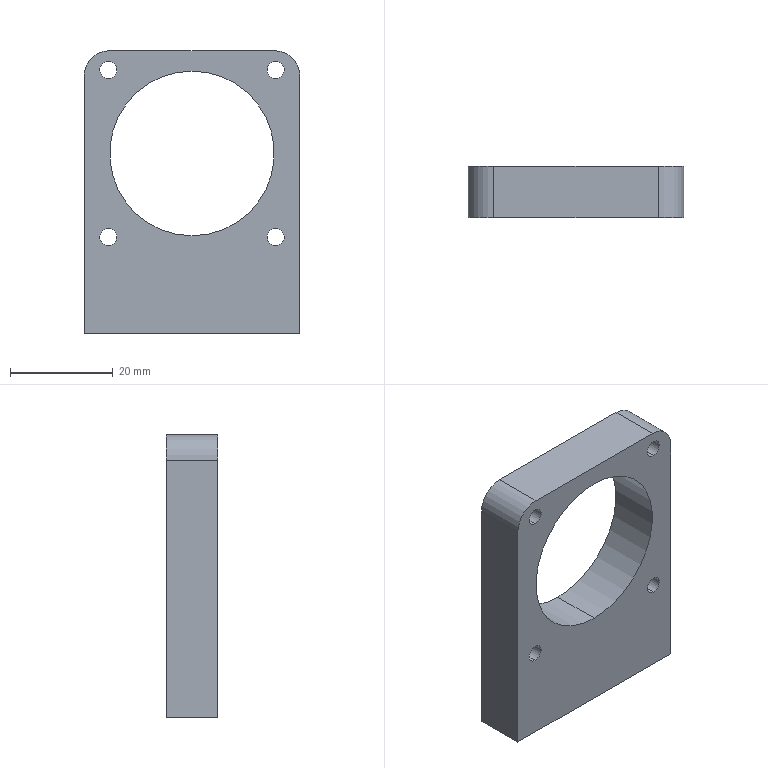Part | 1 solid | 26 faces | box 42 x 10 x 55 mm | volume 14397 mm3 | cylinder 16 | plane 6 | cone 4 | commonest cylinder face diameters 3.3 x12 10 x2 32 x2
STEP:
#1=CARTESIAN_POINT('',(-16.265,-5.,-18.915));
#2=VERTEX_POINT('',#1);
#3=CARTESIAN_POINT('',(-16.265,-5.,-15.615));
#4=VERTEX_POINT('',#3);
#5=CARTESIAN_POINT('',(-16.265,-5.,-17.265));
#6=DIRECTION('',(0.,1.,0.));
#7=DIRECTION('',(0.,0.,1.));
#8=AXIS2_PLACEMENT_3D('',#5,#6,#7);
#9=CIRCLE('',#8,1.65);
#10=EDGE_CURVE('',#2,#4,#9,.T.);
#11=ORIENTED_EDGE('',*,*,#10,.F.);
#12=CARTESIAN_POINT('',(-16.265,5.,-18.915));
#13=VERTEX_POINT('',#12);
#14=CARTESIAN_POINT('',(-16.265,5.,-18.915));
#15=DIRECTION('',(0.,1.,0.));
#16=VECTOR('',#15,1000.);
#17=LINE('',#14,#16);
#18=EDGE_CURVE('',#2,#13,#17,.T.);
#19=ORIENTED_EDGE('',*,*,#18,.T.);
#20=CARTESIAN_POINT('',(-16.265,5.,-15.615));
#21=VERTEX_POINT('',#20);
#22=CARTESIAN_POINT('',(-16.265,5.,-17.265));
#23=DIRECTION('',(0.,1.,0.));
#24=DIRECTION('',(0.,0.,1.));
#25=AXIS2_PLACEMENT_3D('',#22,#23,#24);
#26=CIRCLE('',#25,1.65);
#27=EDGE_CURVE('',#13,#21,#26,.T.);
#28=ORIENTED_EDGE('',*,*,#27,.T.);
#29=CARTESIAN_POINT('',(-16.265,5.,-15.615));
#30=DIRECTION('',(0.,1.,0.));
#31=VECTOR('',#30,1000.);
#32=LINE('',#29,#31);
#33=EDGE_CURVE('',#4,#21,#32,.T.);
#34=ORIENTED_EDGE('',*,*,#33,.F.);
#35=EDGE_LOOP('',(#11,#19,#28,#34));
#36=FACE_OUTER_BOUND('',#35,.T.);
#37=CARTESIAN_POINT('',(-16.265,5.,-17.265));
#38=DIRECTION('',(0.,1.,0.));
#39=DIRECTION('',(0.,0.,1.));
#40=AXIS2_PLACEMENT_3D('',#37,#38,#39);
#41=CYLINDRICAL_SURFACE('',#40,1.65);
#42=ADVANCED_FACE('',(#36),#41,.F.);
#43=CARTESIAN_POINT('',(16.265,-5.,-18.915));
#44=VERTEX_POINT('',#43);
#45=CARTESIAN_POINT('',(16.265,-5.,-15.615));
#46=VERTEX_POINT('',#45);
#47=CARTESIAN_POINT('',(16.265,-5.,-17.265));
#48=DIRECTION('',(0.,1.,0.));
#49=DIRECTION('',(0.,0.,1.));
#50=AXIS2_PLACEMENT_3D('',#47,#48,#49);
#51=CIRCLE('',#50,1.65);
#52=EDGE_CURVE('',#44,#46,#51,.T.);
#53=ORIENTED_EDGE('',*,*,#52,.F.);
#54=CARTESIAN_POINT('',(16.265,5.,-18.915));
#55=VERTEX_POINT('',#54);
#56=CARTESIAN_POINT('',(16.265,5.,-18.915));
#57=DIRECTION('',(0.,1.,0.));
#58=VECTOR('',#57,1000.);
#59=LINE('',#56,#58);
#60=EDGE_CURVE('',#44,#55,#59,.T.);
#61=ORIENTED_EDGE('',*,*,#60,.T.);
#62=CARTESIAN_POINT('',(16.265,5.,-15.615));
#63=VERTEX_POINT('',#62);
#64=CARTESIAN_POINT('',(16.265,5.,-17.265));
#65=DIRECTION('',(0.,1.,0.));
#66=DIRECTION('',(0.,0.,1.));
#67=AXIS2_PLACEMENT_3D('',#64,#65,#66);
#68=CIRCLE('',#67,1.65);
#69=EDGE_CURVE('',#55,#63,#68,.T.);
#70=ORIENTED_EDGE('',*,*,#69,.T.);
#71=CARTESIAN_POINT('',(16.265,5.,-15.615));
#72=DIRECTION('',(0.,1.,0.));
#73=VECTOR('',#72,1000.);
#74=LINE('',#71,#73);
#75=EDGE_CURVE('',#46,#63,#74,.T.);
#76=ORIENTED_EDGE('',*,*,#75,.F.);
#77=EDGE_LOOP('',(#53,#61,#70,#76));
#78=FACE_OUTER_BOUND('',#77,.T.);
#79=CARTESIAN_POINT('',(16.265,5.,-17.265));
#80=DIRECTION('',(0.,1.,0.));
#81=DIRECTION('',(0.,0.,1.));
#82=AXIS2_PLACEMENT_3D('',#79,#80,#81);
#83=CYLINDRICAL_SURFACE('',#82,1.65);
#84=ADVANCED_FACE('',(#78),#83,.F.);
#85=CARTESIAN_POINT('',(-16.265,-5.,13.615));
#86=VERTEX_POINT('',#85);
#87=CARTESIAN_POINT('',(-16.265,-5.,16.915));
#88=VERTEX_POINT('',#87);
#89=CARTESIAN_POINT('',(-16.265,-5.,15.265));
#90=DIRECTION('',(0.,1.,0.));
#91=DIRECTION('',(0.,0.,1.));
#92=AXIS2_PLACEMENT_3D('',#89,#90,#91);
#93=CIRCLE('',#92,1.65);
#94=EDGE_CURVE('',#86,#88,#93,.T.);
#95=ORIENTED_EDGE('',*,*,#94,.F.);
#96=CARTESIAN_POINT('',(-16.265,5.,13.615));
#97=VERTEX_POINT('',#96);
#98=CARTESIAN_POINT('',(-16.265,5.,13.615));
#99=DIRECTION('',(0.,1.,0.));
#100=VECTOR('',#99,1000.);
#101=LINE('',#98,#100);
#102=EDGE_CURVE('',#86,#97,#101,.T.);
#103=ORIENTED_EDGE('',*,*,#102,.T.);
#104=CARTESIAN_POINT('',(-16.265,5.,16.915));
#105=VERTEX_POINT('',#104);
#106=CARTESIAN_POINT('',(-16.265,5.,15.265));
#107=DIRECTION('',(0.,1.,0.));
#108=DIRECTION('',(0.,0.,1.));
#109=AXIS2_PLACEMENT_3D('',#106,#107,#108);
#110=CIRCLE('',#109,1.65);
#111=EDGE_CURVE('',#97,#105,#110,.T.);
#112=ORIENTED_EDGE('',*,*,#111,.T.);
#113=CARTESIAN_POINT('',(-16.265,5.,16.915));
#114=DIRECTION('',(0.,1.,0.));
#115=VECTOR('',#114,1000.);
#116=LINE('',#113,#115);
#117=EDGE_CURVE('',#88,#105,#116,.T.);
#118=ORIENTED_EDGE('',*,*,#117,.F.);
#119=EDGE_LOOP('',(#95,#103,#112,#118));
#120=FACE_OUTER_BOUND('',#119,.T.);
#121=CARTESIAN_POINT('',(-16.265,5.,15.265));
#122=DIRECTION('',(0.,1.,0.));
#123=DIRECTION('',(0.,0.,1.));
#124=AXIS2_PLACEMENT_3D('',#121,#122,#123);
#125=CYLINDRICAL_SURFACE('',#124,1.65);
#126=ADVANCED_FACE('',(#120),#125,.F.);
#127=CARTESIAN_POINT('',(16.265,-5.,13.615));
#128=VERTEX_POINT('',#127);
#129=CARTESIAN_POINT('',(16.265,-5.,16.915));
#130=VERTEX_POINT('',#129);
#131=CARTESIAN_POINT('',(16.265,-5.,15.265));
#132=DIRECTION('',(0.,1.,0.));
#133=DIRECTION('',(0.,0.,1.));
#134=AXIS2_PLACEMENT_3D('',#131,#132,#133);
#135=CIRCLE('',#134,1.65);
#136=EDGE_CURVE('',#128,#130,#135,.T.);
#137=ORIENTED_EDGE('',*,*,#136,.F.);
#138=CARTESIAN_POINT('',(16.265,5.,13.615));
#139=VERTEX_POINT('',#138);
#140=CARTESIAN_POINT('',(16.265,5.,13.615));
#141=DIRECTION('',(0.,1.,0.));
#142=VECTOR('',#141,1000.);
#143=LINE('',#140,#142);
#144=EDGE_CURVE('',#128,#139,#143,.T.);
#145=ORIENTED_EDGE('',*,*,#144,.T.);
#146=CARTESIAN_POINT('',(16.265,5.,16.915));
#147=VERTEX_POINT('',#146);
#148=CARTESIAN_POINT('',(16.265,5.,15.265));
#149=DIRECTION('',(0.,1.,0.));
#150=DIRECTION('',(0.,0.,1.));
#151=AXIS2_PLACEMENT_3D('',#148,#149,#150);
#152=CIRCLE('',#151,1.65);
#153=EDGE_CURVE('',#139,#147,#152,.T.);
#154=ORIENTED_EDGE('',*,*,#153,.T.);
#155=CARTESIAN_POINT('',(16.265,5.,16.915));
#156=DIRECTION('',(0.,1.,0.));
#157=VECTOR('',#156,1000.);
#158=LINE('',#155,#157);
#159=EDGE_CURVE('',#130,#147,#158,.T.);
#160=ORIENTED_EDGE('',*,*,#159,.F.);
#161=EDGE_LOOP('',(#137,#145,#154,#160));
#162=FACE_OUTER_BOUND('',#161,.T.);
#163=CARTESIAN_POINT('',(16.265,5.,15.265));
#164=DIRECTION('',(0.,1.,0.));
#165=DIRECTION('',(0.,0.,1.));
#166=AXIS2_PLACEMENT_3D('',#163,#164,#165);
#167=CYLINDRICAL_SURFACE('',#166,1.65);
#168=ADVANCED_FACE('',(#162),#167,.F.);
#169=CARTESIAN_POINT('',(0.,-5.,-17.));
#170=VERTEX_POINT('',#169);
#171=CARTESIAN_POINT('',(0.,-5.,15.));
#172=VERTEX_POINT('',#171);
#173=CARTESIAN_POINT('',(0.,-5.,-1.));
#174=DIRECTION('',(0.,1.,0.));
#175=DIRECTION('',(0.,0.,1.));
#176=AXIS2_PLACEMENT_3D('',#173,#174,#175);
#177=CIRCLE('',#176,16.);
#178=EDGE_CURVE('',#170,#172,#177,.T.);
#179=ORIENTED_EDGE('',*,*,#178,.F.);
#180=CARTESIAN_POINT('',(0.,5.,-17.));
#181=VERTEX_POINT('',#180);
#182=CARTESIAN_POINT('',(0.,-5.,-17.));
#183=DIRECTION('',(0.,1.,0.));
#184=VECTOR('',#183,1000.);
#185=LINE('',#182,#184);
#186=EDGE_CURVE('',#170,#181,#185,.T.);
#187=ORIENTED_EDGE('',*,*,#186,.T.);
#188=CARTESIAN_POINT('',(0.,5.,15.));
#189=VERTEX_POINT('',#188);
#190=CARTESIAN_POINT('',(0.,5.,-1.));
#191=DIRECTION('',(0.,1.,0.));
#192=DIRECTION('',(0.,0.,1.));
#193=AXIS2_PLACEMENT_3D('',#190,#191,#192);
#194=CIRCLE('',#193,16.);
#195=EDGE_CURVE('',#181,#189,#194,.T.);
#196=ORIENTED_EDGE('',*,*,#195,.T.);
#197=CARTESIAN_POINT('',(0.,-5.,15.));
#198=DIRECTION('',(0.,1.,0.));
#199=VECTOR('',#198,1000.);
#200=LINE('',#197,#199);
#201=EDGE_CURVE('',#172,#189,#200,.T.);
#202=ORIENTED_EDGE('',*,*,#201,.F.);
#203=EDGE_LOOP('',(#179,#187,#196,#202));
#204=FACE_OUTER_BOUND('',#203,.T.);
#205=CARTESIAN_POINT('',(0.,-5.,-1.));
#206=DIRECTION('',(0.,1.,0.));
#207=DIRECTION('',(0.,0.,1.));
#208=AXIS2_PLACEMENT_3D('',#205,#206,#207);
#209=CYLINDRICAL_SURFACE('',#208,16.);
#210=ADVANCED_FACE('',(#204),#209,.F.);
#211=CARTESIAN_POINT('',(16.65,0.,-24.));
#212=VERTEX_POINT('',#211);
#213=CARTESIAN_POINT('',(13.35,0.,-24.));
#214=VERTEX_POINT('',#213);
#215=CARTESIAN_POINT('',(15.,0.,-24.));
#216=DIRECTION('',(0.,0.,-1.));
#217=DIRECTION('',(-1.,0.,0.));
#218=AXIS2_PLACEMENT_3D('',#215,#216,#217);
#219=CIRCLE('',#218,1.65);
#220=EDGE_CURVE('',#212,#214,#219,.T.);
#221=ORIENTED_EDGE('',*,*,#220,.F.);
#222=CARTESIAN_POINT('',(16.65,0.,-36.));
#223=VERTEX_POINT('',#222);
#224=CARTESIAN_POINT('',(16.65,0.,-36.));
#225=DIRECTION('',(0.,0.,-1.));
#226=VECTOR('',#225,1000.);
#227=LINE('',#224,#226);
#228=EDGE_CURVE('',#212,#223,#227,.T.);
#229=ORIENTED_EDGE('',*,*,#228,.T.);
#230=CARTESIAN_POINT('',(13.35,0.,-36.));
#231=VERTEX_POINT('',#230);
#232=CARTESIAN_POINT('',(15.,0.,-36.));
#233=DIRECTION('',(0.,0.,-1.));
#234=DIRECTION('',(-1.,0.,0.));
#235=AXIS2_PLACEMENT_3D('',#232,#233,#234);
#236=CIRCLE('',#235,1.65);
#237=EDGE_CURVE('',#223,#231,#236,.T.);
#238=ORIENTED_EDGE('',*,*,#237,.T.);
#239=CARTESIAN_POINT('',(13.35,0.,-36.));
#240=DIRECTION('',(0.,0.,-1.));
#241=VECTOR('',#240,1000.);
#242=LINE('',#239,#241);
#243=EDGE_CURVE('',#214,#231,#242,.T.);
#244=ORIENTED_EDGE('',*,*,#243,.F.);
#245=EDGE_LOOP('',(#221,#229,#238,#244));
#246=FACE_OUTER_BOUND('',#245,.T.);
#247=CARTESIAN_POINT('',(15.,0.,-36.));
#248=DIRECTION('',(0.,0.,-1.));
#249=DIRECTION('',(-1.,0.,0.));
#250=AXIS2_PLACEMENT_3D('',#247,#248,#249);
#251=CYLINDRICAL_SURFACE('',#250,1.65);
#252=ADVANCED_FACE('',(#246),#251,.F.);
#253=CARTESIAN_POINT('',(15.,0.,-23.009));
#254=VERTEX_POINT('',#253);
#255=CARTESIAN_POINT('',(13.35,0.,-24.));
#256=DIRECTION('',(-0.8572,0.,-0.515));
#257=VECTOR('',#256,1000.);
#258=LINE('',#255,#257);
#259=EDGE_CURVE('',#254,#214,#258,.T.);
#260=ORIENTED_EDGE('',*,*,#259,.F.);
#261=CARTESIAN_POINT('',(16.65,0.,-24.));
#262=DIRECTION('',(0.8572,0.,-0.515));
#263=VECTOR('',#262,1000.);
#264=LINE('',#261,#263);
#265=EDGE_CURVE('',#254,#212,#264,.T.);
#266=ORIENTED_EDGE('',*,*,#265,.T.);
#267=ORIENTED_EDGE('',*,*,#220,.T.);
#268=EDGE_LOOP('',(#260,#266,#267));
#269=FACE_OUTER_BOUND('',#268,.T.);
#270=CARTESIAN_POINT('',(15.,0.,-24.));
#271=DIRECTION('',(0.,0.,-1.));
#272=DIRECTION('',(-1.,0.,0.));
#273=AXIS2_PLACEMENT_3D('',#270,#271,#272);
#274=CONICAL_SURFACE('',#273,1.65,1.03);
#275=ADVANCED_FACE('',(#269),#274,.F.);
#276=CARTESIAN_POINT('',(-13.35,0.,-24.));
#277=VERTEX_POINT('',#276);
#278=CARTESIAN_POINT('',(-16.65,0.,-24.));
#279=VERTEX_POINT('',#278);
#280=CARTESIAN_POINT('',(-15.,0.,-24.));
#281=DIRECTION('',(0.,0.,-1.));
#282=DIRECTION('',(-1.,0.,0.));
#283=AXIS2_PLACEMENT_3D('',#280,#281,#282);
#284=CIRCLE('',#283,1.65);
#285=EDGE_CURVE('',#277,#279,#284,.T.);
#286=ORIENTED_EDGE('',*,*,#285,.F.);
#287=CARTESIAN_POINT('',(-13.35,0.,-36.));
#288=VERTEX_POINT('',#287);
#289=CARTESIAN_POINT('',(-13.35,0.,-36.));
#290=DIRECTION('',(0.,0.,-1.));
#291=VECTOR('',#290,1000.);
#292=LINE('',#289,#291);
#293=EDGE_CURVE('',#277,#288,#292,.T.);
#294=ORIENTED_EDGE('',*,*,#293,.T.);
#295=CARTESIAN_POINT('',(-16.65,0.,-36.));
#296=VERTEX_POINT('',#295);
#297=CARTESIAN_POINT('',(-15.,0.,-36.));
#298=DIRECTION('',(0.,0.,-1.));
#299=DIRECTION('',(-1.,0.,0.));
#300=AXIS2_PLACEMENT_3D('',#297,#298,#299);
#301=CIRCLE('',#300,1.65);
#302=EDGE_CURVE('',#288,#296,#301,.T.);
#303=ORIENTED_EDGE('',*,*,#302,.T.);
#304=CARTESIAN_POINT('',(-16.65,0.,-36.));
#305=DIRECTION('',(0.,0.,-1.));
#306=VECTOR('',#305,1000.);
#307=LINE('',#304,#306);
#308=EDGE_CURVE('',#279,#296,#307,.T.);
#309=ORIENTED_EDGE('',*,*,#308,.F.);
#310=EDGE_LOOP('',(#286,#294,#303,#309));
#311=FACE_OUTER_BOUND('',#310,.T.);
#312=CARTESIAN_POINT('',(-15.,0.,-36.));
#313=DIRECTION('',(0.,0.,-1.));
#314=DIRECTION('',(-1.,0.,0.));
#315=AXIS2_PLACEMENT_3D('',#312,#313,#314);
#316=CYLINDRICAL_SURFACE('',#315,1.65);
#317=ADVANCED_FACE('',(#311),#316,.F.);
#318=CARTESIAN_POINT('',(-15.,0.,-23.009));
#319=VERTEX_POINT('',#318);
#320=CARTESIAN_POINT('',(-16.65,0.,-24.));
#321=DIRECTION('',(-0.8572,0.,-0.515));
#322=VECTOR('',#321,1000.);
#323=LINE('',#320,#322);
#324=EDGE_CURVE('',#319,#279,#323,.T.);
#325=ORIENTED_EDGE('',*,*,#324,.F.);
#326=CARTESIAN_POINT('',(-13.35,0.,-24.));
#327=DIRECTION('',(0.8572,0.,-0.515));
#328=VECTOR('',#327,1000.);
#329=LINE('',#326,#328);
#330=EDGE_CURVE('',#319,#277,#329,.T.);
#331=ORIENTED_EDGE('',*,*,#330,.T.);
#332=ORIENTED_EDGE('',*,*,#285,.T.);
#333=EDGE_LOOP('',(#325,#331,#332));
#334=FACE_OUTER_BOUND('',#333,.T.);
#335=CARTESIAN_POINT('',(-15.,0.,-24.));
#336=DIRECTION('',(0.,0.,-1.));
#337=DIRECTION('',(-1.,0.,0.));
#338=AXIS2_PLACEMENT_3D('',#335,#336,#337);
#339=CONICAL_SURFACE('',#338,1.65,1.03);
#340=ADVANCED_FACE('',(#334),#339,.F.);
#341=CARTESIAN_POINT('',(21.,5.,14.));
#342=VERTEX_POINT('',#341);
#343=CARTESIAN_POINT('',(21.,5.,-36.));
#344=VERTEX_POINT('',#343);
#345=CARTESIAN_POINT('',(21.,5.,-36.));
#346=DIRECTION('',(0.,0.,-1.));
#347=VECTOR('',#346,1000.);
#348=LINE('',#345,#347);
#349=EDGE_CURVE('',#342,#344,#348,.T.);
#350=ORIENTED_EDGE('',*,*,#349,.F.);
#351=CARTESIAN_POINT('',(21.,-5.,14.));
#352=VERTEX_POINT('',#351);
#353=CARTESIAN_POINT('',(21.,5.,14.));
#354=DIRECTION('',(0.,-1.,0.));
#355=VECTOR('',#354,1000.);
#356=LINE('',#353,#355);
#357=EDGE_CURVE('',#342,#352,#356,.T.);
#358=ORIENTED_EDGE('',*,*,#357,.T.);
#359=CARTESIAN_POINT('',(21.,-5.,-36.));
#360=VERTEX_POINT('',#359);
#361=CARTESIAN_POINT('',(21.,-5.,-36.));
#362=DIRECTION('',(0.,0.,-1.));
#363=VECTOR('',#362,1000.);
#364=LINE('',#361,#363);
#365=EDGE_CURVE('',#352,#360,#364,.T.);
#366=ORIENTED_EDGE('',*,*,#365,.T.);
#367=CARTESIAN_POINT('',(21.,5.,-36.));
#368=DIRECTION('',(0.,-1.,0.));
#369=VECTOR('',#368,1000.);
#370=LINE('',#367,#369);
#371=EDGE_CURVE('',#344,#360,#370,.T.);
#372=ORIENTED_EDGE('',*,*,#371,.F.);
#373=EDGE_LOOP('',(#350,#358,#366,#372));
#374=FACE_OUTER_BOUND('',#373,.T.);
#375=CARTESIAN_POINT('',(21.,5.,-36.));
#376=DIRECTION('',(-1.,0.,0.));
#377=DIRECTION('',(0.,0.,1.));
#378=AXIS2_PLACEMENT_3D('',#375,#376,#377);
#379=PLANE('',#378);
#380=ADVANCED_FACE('',(#374),#379,.F.);
#381=CARTESIAN_POINT('',(15.,0.,-36.));
#382=DIRECTION('',(0.,0.,-1.));
#383=DIRECTION('',(-1.,0.,0.));
#384=AXIS2_PLACEMENT_3D('',#381,#382,#383);
#385=CIRCLE('',#384,1.65);
#386=EDGE_CURVE('',#231,#223,#385,.T.);
#387=ORIENTED_EDGE('',*,*,#386,.F.);
#388=ORIENTED_EDGE('',*,*,#237,.F.);
#389=EDGE_LOOP('',(#387,#388));
#390=FACE_BOUND('',#389,.T.);
#391=CARTESIAN_POINT('',(-15.,0.,-36.));
#392=DIRECTION('',(0.,0.,-1.));
#393=DIRECTION('',(-1.,0.,0.));
#394=AXIS2_PLACEMENT_3D('',#391,#392,#393);
#395=CIRCLE('',#394,1.65);
#396=EDGE_CURVE('',#296,#288,#395,.T.);
#397=ORIENTED_EDGE('',*,*,#396,.F.);
#398=ORIENTED_EDGE('',*,*,#302,.F.);
#399=EDGE_LOOP('',(#397,#398));
#400=FACE_BOUND('',#399,.T.);
#401=CARTESIAN_POINT('',(-21.,-5.,-36.));
#402=VERTEX_POINT('',#401);
#403=CARTESIAN_POINT('',(-21.,-5.,-36.));
#404=DIRECTION('',(-1.,0.,0.));
#405=VECTOR('',#404,1000.);
#406=LINE('',#403,#405);
#407=EDGE_CURVE('',#360,#402,#406,.T.);
#408=ORIENTED_EDGE('',*,*,#407,.T.);
#409=CARTESIAN_POINT('',(-21.,5.,-36.));
#410=VERTEX_POINT('',#409);
#411=CARTESIAN_POINT('',(-21.,5.,-36.));
#412=DIRECTION('',(0.,-1.,0.));
#413=VECTOR('',#412,1000.);
#414=LINE('',#411,#413);
#415=EDGE_CURVE('',#410,#402,#414,.T.);
#416=ORIENTED_EDGE('',*,*,#415,.F.);
#417=CARTESIAN_POINT('',(-21.,5.,-36.));
#418=DIRECTION('',(-1.,0.,0.));
#419=VECTOR('',#418,1000.);
#420=LINE('',#417,#419);
#421=EDGE_CURVE('',#344,#410,#420,.T.);
#422=ORIENTED_EDGE('',*,*,#421,.F.);
#423=ORIENTED_EDGE('',*,*,#371,.T.);
#424=EDGE_LOOP('',(#408,#416,#422,#423));
#425=FACE_OUTER_BOUND('',#424,.T.);
#426=CARTESIAN_POINT('',(-21.,5.,-36.));
#427=DIRECTION('',(0.,0.,1.));
#428=DIRECTION('',(1.,0.,0.));
#429=AXIS2_PLACEMENT_3D('',#426,#427,#428);
#430=PLANE('',#429);
#431=ADVANCED_FACE('',(#390,#400,#425),#430,.F.);
#432=CARTESIAN_POINT('',(-21.,-5.,14.));
#433=VERTEX_POINT('',#432);
#434=CARTESIAN_POINT('',(-21.,-5.,-36.));
#435=DIRECTION('',(0.,0.,1.));
#436=VECTOR('',#435,1000.);
#437=LINE('',#434,#436);
#438=EDGE_CURVE('',#402,#433,#437,.T.);
#439=ORIENTED_EDGE('',*,*,#438,.T.);
#440=CARTESIAN_POINT('',(-21.,5.,14.));
#441=VERTEX_POINT('',#440);
#442=CARTESIAN_POINT('',(-21.,5.,14.));
#443=DIRECTION('',(0.,1.,0.));
#444=VECTOR('',#443,1000.);
#445=LINE('',#442,#444);
#446=EDGE_CURVE('',#433,#441,#445,.T.);
#447=ORIENTED_EDGE('',*,*,#446,.T.);
#448=CARTESIAN_POINT('',(-21.,5.,-36.));
#449=DIRECTION('',(0.,0.,1.));
#450=VECTOR('',#449,1000.);
#451=LINE('',#448,#450);
#452=EDGE_CURVE('',#410,#441,#451,.T.);
#453=ORIENTED_EDGE('',*,*,#452,.F.);
#454=ORIENTED_EDGE('',*,*,#415,.T.);
#455=EDGE_LOOP('',(#439,#447,#453,#454));
#456=FACE_OUTER_BOUND('',#455,.T.);
#457=CARTESIAN_POINT('',(-21.,5.,-36.));
#458=DIRECTION('',(1.,0.,0.));
#459=DIRECTION('',(0.,0.,-1.));
#460=AXIS2_PLACEMENT_3D('',#457,#458,#459);
#461=PLANE('',#460);
#462=ADVANCED_FACE('',(#456),#461,.F.);
#463=CARTESIAN_POINT('',(-16.265,5.,-17.265));
#464=DIRECTION('',(0.,1.,0.));
#465=DIRECTION('',(0.,0.,1.));
#466=AXIS2_PLACEMENT_3D('',#463,#464,#465);
#467=CIRCLE('',#466,1.65);
#468=EDGE_CURVE('',#21,#13,#467,.T.);
#469=ORIENTED_EDGE('',*,*,#468,.F.);
#470=ORIENTED_EDGE('',*,*,#27,.F.);
#471=EDGE_LOOP('',(#469,#470));
#472=FACE_BOUND('',#471,.T.);
#473=CARTESIAN_POINT('',(16.265,5.,-17.265));
#474=DIRECTION('',(0.,1.,0.));
#475=DIRECTION('',(0.,0.,1.));
#476=AXIS2_PLACEMENT_3D('',#473,#474,#475);
#477=CIRCLE('',#476,1.65);
#478=EDGE_CURVE('',#63,#55,#477,.T.);
#479=ORIENTED_EDGE('',*,*,#478,.F.);
#480=ORIENTED_EDGE('',*,*,#69,.F.);
#481=EDGE_LOOP('',(#479,#480));
#482=FACE_BOUND('',#481,.T.);
#483=CARTESIAN_POINT('',(-16.265,5.,15.265));
#484=DIRECTION('',(0.,1.,0.));
#485=DIRECTION('',(0.,0.,1.));
#486=AXIS2_PLACEMENT_3D('',#483,#484,#485);
#487=CIRCLE('',#486,1.65);
#488=EDGE_CURVE('',#105,#97,#487,.T.);
#489=ORIENTED_EDGE('',*,*,#488,.F.);
#490=ORIENTED_EDGE('',*,*,#111,.F.);
#491=EDGE_LOOP('',(#489,#490));
#492=FACE_BOUND('',#491,.T.);
#493=CARTESIAN_POINT('',(16.265,5.,15.265));
#494=DIRECTION('',(0.,1.,0.));
#495=DIRECTION('',(0.,0.,1.));
#496=AXIS2_PLACEMENT_3D('',#493,#494,#495);
#497=CIRCLE('',#496,1.65);
#498=EDGE_CURVE('',#147,#139,#497,.T.);
#499=ORIENTED_EDGE('',*,*,#498,.F.);
#500=ORIENTED_EDGE('',*,*,#153,.F.);
#501=EDGE_LOOP('',(#499,#500));
#502=FACE_BOUND('',#501,.T.);
#503=ORIENTED_EDGE('',*,*,#452,.T.);
#504=CARTESIAN_POINT('',(-16.,5.,19.));
#505=VERTEX_POINT('',#504);
#506=CARTESIAN_POINT('',(-16.,5.,14.));
#507=DIRECTION('',(0.,1.,0.));
#508=DIRECTION('',(0.,0.,1.));
#509=AXIS2_PLACEMENT_3D('',#506,#507,#508);
#510=CIRCLE('',#509,5.);
#511=EDGE_CURVE('',#441,#505,#510,.T.);
#512=ORIENTED_EDGE('',*,*,#511,.T.);
#513=CARTESIAN_POINT('',(16.,5.,19.));
#514=VERTEX_POINT('',#513);
#515=CARTESIAN_POINT('',(-32.61,5.,19.));
#516=DIRECTION('',(-1.,0.,0.));
#517=VECTOR('',#516,1000.);
#518=LINE('',#515,#517);
#519=EDGE_CURVE('',#514,#505,#518,.T.);
#520=ORIENTED_EDGE('',*,*,#519,.F.);
#521=CARTESIAN_POINT('',(16.,5.,14.));
#522=DIRECTION('',(0.,1.,0.));
#523=DIRECTION('',(0.,0.,1.));
#524=AXIS2_PLACEMENT_3D('',#521,#522,#523);
#525=CIRCLE('',#524,5.);
#526=EDGE_CURVE('',#514,#342,#525,.T.);
#527=ORIENTED_EDGE('',*,*,#526,.T.);
#528=ORIENTED_EDGE('',*,*,#349,.T.);
#529=ORIENTED_EDGE('',*,*,#421,.T.);
#530=EDGE_LOOP('',(#503,#512,#520,#527,#528,#529));
#531=FACE_OUTER_BOUND('',#530,.T.);
#532=CARTESIAN_POINT('',(0.,5.,-1.));
#533=DIRECTION('',(0.,1.,0.));
#534=DIRECTION('',(0.,0.,1.));
#535=AXIS2_PLACEMENT_3D('',#532,#533,#534);
#536=CIRCLE('',#535,16.);
#537=EDGE_CURVE('',#189,#181,#536,.T.);
#538=ORIENTED_EDGE('',*,*,#537,.F.);
#539=ORIENTED_EDGE('',*,*,#195,.F.);
#540=EDGE_LOOP('',(#538,#539));
#541=FACE_BOUND('',#540,.T.);
#542=CARTESIAN_POINT('',(0.,5.,0.));
#543=DIRECTION('',(0.,1.,0.));
#544=DIRECTION('',(0.,0.,1.));
#545=AXIS2_PLACEMENT_3D('',#542,#543,#544);
#546=PLANE('',#545);
#547=ADVANCED_FACE('',(#472,#482,#492,#502,#531,#541),#546,.T.);
#548=CARTESIAN_POINT('',(-16.265,-5.,-17.265));
#549=DIRECTION('',(0.,1.,0.));
#550=DIRECTION('',(0.,0.,1.));
#551=AXIS2_PLACEMENT_3D('',#548,#549,#550);
#552=CIRCLE('',#551,1.65);
#553=EDGE_CURVE('',#4,#2,#552,.T.);
#554=ORIENTED_EDGE('',*,*,#553,.T.);
#555=ORIENTED_EDGE('',*,*,#10,.T.);
#556=EDGE_LOOP('',(#554,#555));
#557=FACE_BOUND('',#556,.T.);
#558=CARTESIAN_POINT('',(16.265,-5.,-17.265));
#559=DIRECTION('',(0.,1.,0.));
#560=DIRECTION('',(0.,0.,1.));
#561=AXIS2_PLACEMENT_3D('',#558,#559,#560);
#562=CIRCLE('',#561,1.65);
#563=EDGE_CURVE('',#46,#44,#562,.T.);
#564=ORIENTED_EDGE('',*,*,#563,.T.);
#565=ORIENTED_EDGE('',*,*,#52,.T.);
#566=EDGE_LOOP('',(#564,#565));
#567=FACE_BOUND('',#566,.T.);
#568=CARTESIAN_POINT('',(-16.265,-5.,15.265));
#569=DIRECTION('',(0.,1.,0.));
#570=DIRECTION('',(0.,0.,1.));
#571=AXIS2_PLACEMENT_3D('',#568,#569,#570);
#572=CIRCLE('',#571,1.65);
#573=EDGE_CURVE('',#88,#86,#572,.T.);
#574=ORIENTED_EDGE('',*,*,#573,.T.);
#575=ORIENTED_EDGE('',*,*,#94,.T.);
#576=EDGE_LOOP('',(#574,#575));
#577=FACE_BOUND('',#576,.T.);
#578=CARTESIAN_POINT('',(16.265,-5.,15.265));
#579=DIRECTION('',(0.,1.,0.));
#580=DIRECTION('',(0.,0.,1.));
#581=AXIS2_PLACEMENT_3D('',#578,#579,#580);
#582=CIRCLE('',#581,1.65);
#583=EDGE_CURVE('',#130,#128,#582,.T.);
#584=ORIENTED_EDGE('',*,*,#583,.T.);
#585=ORIENTED_EDGE('',*,*,#136,.T.);
#586=EDGE_LOOP('',(#584,#585));
#587=FACE_BOUND('',#586,.T.);
#588=CARTESIAN_POINT('',(0.,-5.,-1.));
#589=DIRECTION('',(0.,1.,0.));
#590=DIRECTION('',(0.,0.,1.));
#591=AXIS2_PLACEMENT_3D('',#588,#589,#590);
#592=CIRCLE('',#591,16.);
#593=EDGE_CURVE('',#172,#170,#592,.T.);
#594=ORIENTED_EDGE('',*,*,#593,.T.);
#595=ORIENTED_EDGE('',*,*,#178,.T.);
#596=EDGE_LOOP('',(#594,#595));
#597=FACE_BOUND('',#596,.T.);
#598=CARTESIAN_POINT('',(16.,-5.,19.));
#599=VERTEX_POINT('',#598);
#600=CARTESIAN_POINT('',(-16.,-5.,19.));
#601=VERTEX_POINT('',#600);
#602=CARTESIAN_POINT('',(0.,-5.,19.));
#603=DIRECTION('',(-1.,0.,0.));
#604=VECTOR('',#603,1000.);
#605=LINE('',#602,#604);
#606=EDGE_CURVE('',#599,#601,#605,.T.);
#607=ORIENTED_EDGE('',*,*,#606,.T.);
#608=CARTESIAN_POINT('',(-16.,-5.,14.));
#609=DIRECTION('',(0.,-1.,0.));
#610=DIRECTION('',(0.,0.,1.));
#611=AXIS2_PLACEMENT_3D('',#608,#609,#610);
#612=CIRCLE('',#611,5.);
#613=EDGE_CURVE('',#601,#433,#612,.T.);
#614=ORIENTED_EDGE('',*,*,#613,.T.);
#615=ORIENTED_EDGE('',*,*,#438,.F.);
#616=ORIENTED_EDGE('',*,*,#407,.F.);
#617=ORIENTED_EDGE('',*,*,#365,.F.);
#618=CARTESIAN_POINT('',(16.,-5.,14.));
#619=DIRECTION('',(0.,-1.,0.));
#620=DIRECTION('',(0.,0.,1.));
#621=AXIS2_PLACEMENT_3D('',#618,#619,#620);
#622=CIRCLE('',#621,5.);
#623=EDGE_CURVE('',#352,#599,#622,.T.);
#624=ORIENTED_EDGE('',*,*,#623,.T.);
#625=EDGE_LOOP('',(#607,#614,#615,#616,#617,#624));
#626=FACE_OUTER_BOUND('',#625,.T.);
#627=CARTESIAN_POINT('',(0.,-5.,0.));
#628=DIRECTION('',(0.,1.,0.));
#629=DIRECTION('',(0.,0.,1.));
#630=AXIS2_PLACEMENT_3D('',#627,#628,#629);
#631=PLANE('',#630);
#632=ADVANCED_FACE('',(#557,#567,#577,#587,#597,#626),#631,.F.);
#633=ORIENTED_EDGE('',*,*,#330,.F.);
#634=ORIENTED_EDGE('',*,*,#324,.T.);
#635=CARTESIAN_POINT('',(-15.,0.,-24.));
#636=DIRECTION('',(0.,0.,-1.));
#637=DIRECTION('',(-1.,0.,0.));
#638=AXIS2_PLACEMENT_3D('',#635,#636,#637);
#639=CIRCLE('',#638,1.65);
#640=EDGE_CURVE('',#279,#277,#639,.T.);
#641=ORIENTED_EDGE('',*,*,#640,.T.);
#642=EDGE_LOOP('',(#633,#634,#641));
#643=FACE_OUTER_BOUND('',#642,.T.);
#644=CARTESIAN_POINT('',(-15.,0.,-24.));
#645=DIRECTION('',(0.,0.,-1.));
#646=DIRECTION('',(-1.,0.,0.));
#647=AXIS2_PLACEMENT_3D('',#644,#645,#646);
#648=CONICAL_SURFACE('',#647,1.65,1.03);
#649=ADVANCED_FACE('',(#643),#648,.F.);
#650=ORIENTED_EDGE('',*,*,#293,.F.);
#651=ORIENTED_EDGE('',*,*,#640,.F.);
#652=ORIENTED_EDGE('',*,*,#308,.T.);
#653=ORIENTED_EDGE('',*,*,#396,.T.);
#654=EDGE_LOOP('',(#650,#651,#652,#653));
#655=FACE_OUTER_BOUND('',#654,.T.);
#656=CARTESIAN_POINT('',(-15.,0.,-36.));
#657=DIRECTION('',(0.,0.,-1.));
#658=DIRECTION('',(-1.,0.,0.));
#659=AXIS2_PLACEMENT_3D('',#656,#657,#658);
#660=CYLINDRICAL_SURFACE('',#659,1.65);
#661=ADVANCED_FACE('',(#655),#660,.F.);
#662=ORIENTED_EDGE('',*,*,#265,.F.);
#663=ORIENTED_EDGE('',*,*,#259,.T.);
#664=CARTESIAN_POINT('',(15.,0.,-24.));
#665=DIRECTION('',(0.,0.,-1.));
#666=DIRECTION('',(-1.,0.,0.));
#667=AXIS2_PLACEMENT_3D('',#664,#665,#666);
#668=CIRCLE('',#667,1.65);
#669=EDGE_CURVE('',#214,#212,#668,.T.);
#670=ORIENTED_EDGE('',*,*,#669,.T.);
#671=EDGE_LOOP('',(#662,#663,#670));
#672=FACE_OUTER_BOUND('',#671,.T.);
#673=CARTESIAN_POINT('',(15.,0.,-24.));
#674=DIRECTION('',(0.,0.,-1.));
#675=DIRECTION('',(-1.,0.,0.));
#676=AXIS2_PLACEMENT_3D('',#673,#674,#675);
#677=CONICAL_SURFACE('',#676,1.65,1.03);
#678=ADVANCED_FACE('',(#672),#677,.F.);
#679=ORIENTED_EDGE('',*,*,#228,.F.);
#680=ORIENTED_EDGE('',*,*,#669,.F.);
#681=ORIENTED_EDGE('',*,*,#243,.T.);
#682=ORIENTED_EDGE('',*,*,#386,.T.);
#683=EDGE_LOOP('',(#679,#680,#681,#682));
#684=FACE_OUTER_BOUND('',#683,.T.);
#685=CARTESIAN_POINT('',(15.,0.,-36.));
#686=DIRECTION('',(0.,0.,-1.));
#687=DIRECTION('',(-1.,0.,0.));
#688=AXIS2_PLACEMENT_3D('',#685,#686,#687);
#689=CYLINDRICAL_SURFACE('',#688,1.65);
#690=ADVANCED_FACE('',(#684),#689,.F.);
#691=ORIENTED_EDGE('',*,*,#186,.F.);
#692=ORIENTED_EDGE('',*,*,#593,.F.);
#693=ORIENTED_EDGE('',*,*,#201,.T.);
#694=ORIENTED_EDGE('',*,*,#537,.T.);
#695=EDGE_LOOP('',(#691,#692,#693,#694));
#696=FACE_OUTER_BOUND('',#695,.T.);
#697=CARTESIAN_POINT('',(0.,-5.,-1.));
#698=DIRECTION('',(0.,1.,0.));
#699=DIRECTION('',(0.,0.,1.));
#700=AXIS2_PLACEMENT_3D('',#697,#698,#699);
#701=CYLINDRICAL_SURFACE('',#700,16.);
#702=ADVANCED_FACE('',(#696),#701,.F.);
#703=ORIENTED_EDGE('',*,*,#519,.T.);
#704=CARTESIAN_POINT('',(-16.,-26.,19.));
#705=DIRECTION('',(0.,-1.,0.));
#706=VECTOR('',#705,1000.);
#707=LINE('',#704,#706);
#708=EDGE_CURVE('',#505,#601,#707,.T.);
#709=ORIENTED_EDGE('',*,*,#708,.T.);
#710=ORIENTED_EDGE('',*,*,#606,.F.);
#711=CARTESIAN_POINT('',(16.,-26.,19.));
#712=DIRECTION('',(0.,1.,0.));
#713=VECTOR('',#712,1000.);
#714=LINE('',#711,#713);
#715=EDGE_CURVE('',#599,#514,#714,.T.);
#716=ORIENTED_EDGE('',*,*,#715,.T.);
#717=EDGE_LOOP('',(#703,#709,#710,#716));
#718=FACE_OUTER_BOUND('',#717,.T.);
#719=CARTESIAN_POINT('',(-32.61,-26.,19.));
#720=DIRECTION('',(0.,0.,-1.));
#721=DIRECTION('',(-1.,0.,0.));
#722=AXIS2_PLACEMENT_3D('',#719,#720,#721);
#723=PLANE('',#722);
#724=ADVANCED_FACE('',(#718),#723,.F.);
#725=ORIENTED_EDGE('',*,*,#613,.F.);
#726=ORIENTED_EDGE('',*,*,#708,.F.);
#727=ORIENTED_EDGE('',*,*,#511,.F.);
#728=ORIENTED_EDGE('',*,*,#446,.F.);
#729=EDGE_LOOP('',(#725,#726,#727,#728));
#730=FACE_OUTER_BOUND('',#729,.T.);
#731=CARTESIAN_POINT('',(-16.,5.,14.));
#732=DIRECTION('',(0.,1.,0.));
#733=DIRECTION('',(0.,0.,1.));
#734=AXIS2_PLACEMENT_3D('',#731,#732,#733);
#735=CYLINDRICAL_SURFACE('',#734,5.);
#736=ADVANCED_FACE('',(#730),#735,.T.);
#737=ORIENTED_EDGE('',*,*,#526,.F.);
#738=ORIENTED_EDGE('',*,*,#715,.F.);
#739=ORIENTED_EDGE('',*,*,#623,.F.);
#740=ORIENTED_EDGE('',*,*,#357,.F.);
#741=EDGE_LOOP('',(#737,#738,#739,#740));
#742=FACE_OUTER_BOUND('',#741,.T.);
#743=CARTESIAN_POINT('',(16.,5.,14.));
#744=DIRECTION('',(0.,-1.,0.));
#745=DIRECTION('',(0.,0.,-1.));
#746=AXIS2_PLACEMENT_3D('',#743,#744,#745);
#747=CYLINDRICAL_SURFACE('',#746,5.);
#748=ADVANCED_FACE('',(#742),#747,.T.);
#749=ORIENTED_EDGE('',*,*,#144,.F.);
#750=ORIENTED_EDGE('',*,*,#583,.F.);
#751=ORIENTED_EDGE('',*,*,#159,.T.);
#752=ORIENTED_EDGE('',*,*,#498,.T.);
#753=EDGE_LOOP('',(#749,#750,#751,#752));
#754=FACE_OUTER_BOUND('',#753,.T.);
#755=CARTESIAN_POINT('',(16.265,5.,15.265));
#756=DIRECTION('',(0.,1.,0.));
#757=DIRECTION('',(0.,0.,1.));
#758=AXIS2_PLACEMENT_3D('',#755,#756,#757);
#759=CYLINDRICAL_SURFACE('',#758,1.65);
#760=ADVANCED_FACE('',(#754),#759,.F.);
#761=ORIENTED_EDGE('',*,*,#102,.F.);
#762=ORIENTED_EDGE('',*,*,#573,.F.);
#763=ORIENTED_EDGE('',*,*,#117,.T.);
#764=ORIENTED_EDGE('',*,*,#488,.T.);
#765=EDGE_LOOP('',(#761,#762,#763,#764));
#766=FACE_OUTER_BOUND('',#765,.T.);
#767=CARTESIAN_POINT('',(-16.265,5.,15.265));
#768=DIRECTION('',(0.,1.,0.));
#769=DIRECTION('',(0.,0.,1.));
#770=AXIS2_PLACEMENT_3D('',#767,#768,#769);
#771=CYLINDRICAL_SURFACE('',#770,1.65);
#772=ADVANCED_FACE('',(#766),#771,.F.);
#773=ORIENTED_EDGE('',*,*,#60,.F.);
#774=ORIENTED_EDGE('',*,*,#563,.F.);
#775=ORIENTED_EDGE('',*,*,#75,.T.);
#776=ORIENTED_EDGE('',*,*,#478,.T.);
#777=EDGE_LOOP('',(#773,#774,#775,#776));
#778=FACE_OUTER_BOUND('',#777,.T.);
#779=CARTESIAN_POINT('',(16.265,5.,-17.265));
#780=DIRECTION('',(0.,1.,0.));
#781=DIRECTION('',(0.,0.,1.));
#782=AXIS2_PLACEMENT_3D('',#779,#780,#781);
#783=CYLINDRICAL_SURFACE('',#782,1.65);
#784=ADVANCED_FACE('',(#778),#783,.F.);
#785=ORIENTED_EDGE('',*,*,#18,.F.);
#786=ORIENTED_EDGE('',*,*,#553,.F.);
#787=ORIENTED_EDGE('',*,*,#33,.T.);
#788=ORIENTED_EDGE('',*,*,#468,.T.);
#789=EDGE_LOOP('',(#785,#786,#787,#788));
#790=FACE_OUTER_BOUND('',#789,.T.);
#791=CARTESIAN_POINT('',(-16.265,5.,-17.265));
#792=DIRECTION('',(0.,1.,0.));
#793=DIRECTION('',(0.,0.,1.));
#794=AXIS2_PLACEMENT_3D('',#791,#792,#793);
#795=CYLINDRICAL_SURFACE('',#794,1.65);
#796=ADVANCED_FACE('',(#790),#795,.F.);
#797=CLOSED_SHELL('',(#42,#84,#126,#168,#210,#252,#275,#317,#340,#380,#431,#462,#547,#632,#649,#661,#678,#690,#702,#724,#736,#748,#760,#772,#784,#796));
#798=MANIFOLD_SOLID_BREP('',#797);
#799=CARTESIAN_POINT('',(0.,0.,0.));
#800=DIRECTION('',(0.,0.,1.));
#801=DIRECTION('',(1.,0.,0.));
#802=AXIS2_PLACEMENT_3D('',#799,#800,#801);
#803=(LENGTH_UNIT()NAMED_UNIT(*)SI_UNIT(.MILLI.,.METRE.));
#804=UNCERTAINTY_MEASURE_WITH_UNIT(LENGTH_MEASURE(0.00001),#803,'','');
#805=(NAMED_UNIT(*)PLANE_ANGLE_UNIT()SI_UNIT($,.RADIAN.));
#806=(NAMED_UNIT(*)SI_UNIT($,.STERADIAN.)SOLID_ANGLE_UNIT());
#807=(GEOMETRIC_REPRESENTATION_CONTEXT(3)GLOBAL_UNCERTAINTY_ASSIGNED_CONTEXT((#804))GLOBAL_UNIT_ASSIGNED_CONTEXT((#803,#805,#806))REPRESENTATION_CONTEXT('',''));
#808=ADVANCED_BREP_SHAPE_REPRESENTATION('',(#798,#802),#807);